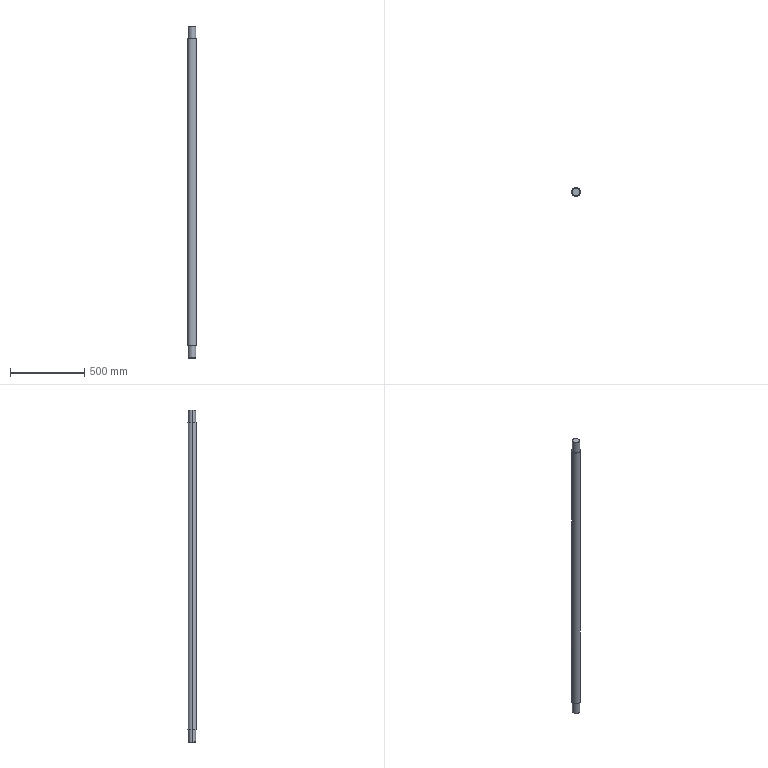Part | SolidWorks | features ICE 2, Chamfer 1, Extrusion 1, MirrorPattern 1 | 1 solid | 26 faces | box 60 x 60 x 2235 mm | volume 6164294 mm3 | cylinder 12 | plane 10 | cone 4 | commonest cylinder face diameters 14 x6 50 x4 60 x2
STEP:
#1=CARTESIAN_POINT('',(7.,24.,-1102.5));
#2=VERTEX_POINT('',#1);
#3=CARTESIAN_POINT('',(0.,25.,-1109.5));
#4=VERTEX_POINT('',#3);
#5=CARTESIAN_POINT('',(7.,24.,-1102.5));
#6=CARTESIAN_POINT('',(7.,24.,-1102.965));
#7=CARTESIAN_POINT('',(6.954,24.014,-1103.422));
#8=CARTESIAN_POINT('',(6.82,24.052,-1104.096));
#9=CARTESIAN_POINT('',(6.764,24.068,-1104.318));
#10=CARTESIAN_POINT('',(6.629,24.105,-1104.759));
#11=CARTESIAN_POINT('',(6.551,24.127,-1104.978));
#12=CARTESIAN_POINT('',(6.287,24.197,-1105.613));
#13=CARTESIAN_POINT('',(6.071,24.253,-1106.014));
#14=CARTESIAN_POINT('',(5.69,24.344,-1106.583));
#15=CARTESIAN_POINT('',(5.552,24.376,-1106.769));
#16=CARTESIAN_POINT('',(5.261,24.441,-1107.123));
#17=CARTESIAN_POINT('',(5.108,24.473,-1107.291));
#18=CARTESIAN_POINT('',(4.626,24.57,-1107.773));
#19=CARTESIAN_POINT('',(4.275,24.635,-1108.062));
#20=CARTESIAN_POINT('',(3.51,24.755,-1108.574));
#21=CARTESIAN_POINT('',(3.106,24.81,-1108.79));
#22=CARTESIAN_POINT('',(2.475,24.878,-1109.052));
#23=CARTESIAN_POINT('',(2.26,24.899,-1109.129));
#24=CARTESIAN_POINT('',(1.82,24.935,-1109.263));
#25=CARTESIAN_POINT('',(1.594,24.95,-1109.32));
#26=CARTESIAN_POINT('',(0.9153,24.987,-1109.455));
#27=CARTESIAN_POINT('',(0.4594,25.,-1109.5));
#28=CARTESIAN_POINT('',(0.,25.,-1109.5));
#29=B_SPLINE_CURVE_WITH_KNOTS('',3,(#5,#6,#7,#8,#9,#10,#11,#12,#13,#14,#15,#16,#17,#18,#19,#20,#21,#22,#23,#24,#25,#26,#27,#28),.UNSPECIFIED.,.F.,.F.,(4,2,2,2,2,2,2,2,2,2,2,4),(0.,0.001375,0.002063,0.00275,0.004125,0.004813,0.0055,0.006875,0.00825,0.008938,0.009626,0.011),.UNSPECIFIED.);
#30=EDGE_CURVE('',#2,#4,#29,.T.);
#31=ORIENTED_EDGE('',*,*,#30,.T.);
#32=CARTESIAN_POINT('',(0.,19.5,-1109.5));
#33=VERTEX_POINT('',#32);
#34=CARTESIAN_POINT('',(0.,25.,-1109.5));
#35=DIRECTION('',(0.,-1.,0.));
#36=VECTOR('',#35,1000.);
#37=LINE('',#34,#36);
#38=EDGE_CURVE('',#4,#33,#37,.T.);
#39=ORIENTED_EDGE('',*,*,#38,.T.);
#40=CARTESIAN_POINT('',(7.,19.5,-1102.5));
#41=VERTEX_POINT('',#40);
#42=CARTESIAN_POINT('',(0.,19.5,-1102.5));
#43=DIRECTION('',(0.,-1.,0.));
#44=DIRECTION('',(0.,0.,1.));
#45=AXIS2_PLACEMENT_3D('',#42,#43,#44);
#46=CIRCLE('',#45,7.);
#47=EDGE_CURVE('',#33,#41,#46,.T.);
#48=ORIENTED_EDGE('',*,*,#47,.T.);
#49=CARTESIAN_POINT('',(7.,25.,-1102.5));
#50=DIRECTION('',(0.,-1.,0.));
#51=VECTOR('',#50,1000.);
#52=LINE('',#49,#51);
#53=EDGE_CURVE('',#2,#41,#52,.T.);
#54=ORIENTED_EDGE('',*,*,#53,.F.);
#55=EDGE_LOOP('',(#31,#39,#48,#54));
#56=FACE_OUTER_BOUND('',#55,.T.);
#57=CARTESIAN_POINT('',(0.,25.,-1102.5));
#58=DIRECTION('',(0.,-1.,0.));
#59=DIRECTION('',(0.,0.,-1.));
#60=AXIS2_PLACEMENT_3D('',#57,#58,#59);
#61=CYLINDRICAL_SURFACE('',#60,7.);
#62=ADVANCED_FACE('',(#56),#61,.F.);
#63=CARTESIAN_POINT('',(-24.,0.,-1117.5));
#64=VERTEX_POINT('',#63);
#65=CARTESIAN_POINT('',(24.,0.,-1117.5));
#66=VERTEX_POINT('',#65);
#67=CARTESIAN_POINT('',(0.,0.,-1117.5));
#68=DIRECTION('',(0.,0.,-1.));
#69=DIRECTION('',(-1.,0.,0.));
#70=AXIS2_PLACEMENT_3D('',#67,#68,#69);
#71=CIRCLE('',#70,24.);
#72=EDGE_CURVE('',#64,#66,#71,.T.);
#73=ORIENTED_EDGE('',*,*,#72,.F.);
#74=CARTESIAN_POINT('',(-25.,0.,-1116.5));
#75=VERTEX_POINT('',#74);
#76=CARTESIAN_POINT('',(-25.,0.,-1116.5));
#77=DIRECTION('',(-0.7071,0.,0.7071));
#78=VECTOR('',#77,1000.);
#79=LINE('',#76,#78);
#80=EDGE_CURVE('',#64,#75,#79,.T.);
#81=ORIENTED_EDGE('',*,*,#80,.T.);
#82=CARTESIAN_POINT('',(25.,0.,-1116.5));
#83=VERTEX_POINT('',#82);
#84=CARTESIAN_POINT('',(0.,0.,-1116.5));
#85=DIRECTION('',(0.,0.,1.));
#86=DIRECTION('',(-1.,0.,0.));
#87=AXIS2_PLACEMENT_3D('',#84,#85,#86);
#88=CIRCLE('',#87,25.);
#89=EDGE_CURVE('',#83,#75,#88,.T.);
#90=ORIENTED_EDGE('',*,*,#89,.F.);
#91=CARTESIAN_POINT('',(25.,0.,-1116.5));
#92=DIRECTION('',(0.7071,0.,0.7071));
#93=VECTOR('',#92,1000.);
#94=LINE('',#91,#93);
#95=EDGE_CURVE('',#66,#83,#94,.T.);
#96=ORIENTED_EDGE('',*,*,#95,.F.);
#97=EDGE_LOOP('',(#73,#81,#90,#96));
#98=FACE_OUTER_BOUND('',#97,.T.);
#99=CARTESIAN_POINT('',(0.,0.,-1116.5));
#100=DIRECTION('',(0.,0.,1.));
#101=DIRECTION('',(1.,0.,0.));
#102=AXIS2_PLACEMENT_3D('',#99,#100,#101);
#103=CONICAL_SURFACE('',#102,25.,0.7854);
#104=ADVANCED_FACE('',(#98),#103,.T.);
#105=ORIENTED_EDGE('',*,*,#30,.F.);
#106=CARTESIAN_POINT('',(7.,24.,-1046.5));
#107=VERTEX_POINT('',#106);
#108=CARTESIAN_POINT('',(7.,24.,-1117.5));
#109=DIRECTION('',(0.,0.,-1.));
#110=VECTOR('',#109,1000.);
#111=LINE('',#108,#110);
#112=EDGE_CURVE('',#107,#2,#111,.T.);
#113=ORIENTED_EDGE('',*,*,#112,.F.);
#114=CARTESIAN_POINT('',(-7.,24.,-1046.5));
#115=VERTEX_POINT('',#114);
#116=CARTESIAN_POINT('',(-7.,24.,-1046.5));
#117=CARTESIAN_POINT('',(-7.,24.,-1046.035));
#118=CARTESIAN_POINT('',(-6.954,24.014,-1045.579));
#119=CARTESIAN_POINT('',(-6.82,24.052,-1044.905));
#120=CARTESIAN_POINT('',(-6.764,24.068,-1044.683));
#121=CARTESIAN_POINT('',(-6.63,24.105,-1044.242));
#122=CARTESIAN_POINT('',(-6.551,24.126,-1044.024));
#123=CARTESIAN_POINT('',(-6.287,24.197,-1043.389));
#124=CARTESIAN_POINT('',(-6.072,24.253,-1042.988));
#125=CARTESIAN_POINT('',(-5.692,24.344,-1042.419));
#126=CARTESIAN_POINT('',(-5.554,24.376,-1042.233));
#127=CARTESIAN_POINT('',(-5.263,24.44,-1041.88));
#128=CARTESIAN_POINT('',(-5.11,24.473,-1041.711));
#129=CARTESIAN_POINT('',(-4.629,24.57,-1041.229));
#130=CARTESIAN_POINT('',(-4.278,24.634,-1040.94));
#131=CARTESIAN_POINT('',(-3.514,24.755,-1040.429));
#132=CARTESIAN_POINT('',(-3.11,24.809,-1040.213));
#133=CARTESIAN_POINT('',(-2.48,24.878,-1039.95));
#134=CARTESIAN_POINT('',(-2.265,24.898,-1039.873));
#135=CARTESIAN_POINT('',(-1.825,24.934,-1039.738));
#136=CARTESIAN_POINT('',(-1.6,24.95,-1039.681));
#137=CARTESIAN_POINT('',(-0.9213,24.987,-1039.546));
#138=CARTESIAN_POINT('',(-0.4657,25.,-1039.5));
#139=CARTESIAN_POINT('',(0.4524,25.,-1039.5));
#140=CARTESIAN_POINT('',(0.9188,24.987,-1039.545));
#141=CARTESIAN_POINT('',(1.818,24.938,-1039.725));
#142=CARTESIAN_POINT('',(2.256,24.902,-1039.858));
#143=CARTESIAN_POINT('',(2.894,24.833,-1040.122));
#144=CARTESIAN_POINT('',(3.103,24.808,-1040.221));
#145=CARTESIAN_POINT('',(3.506,24.754,-1040.437));
#146=CARTESIAN_POINT('',(3.701,24.725,-1040.554));
#147=CARTESIAN_POINT('',(4.079,24.666,-1040.807));
#148=CARTESIAN_POINT('',(4.262,24.635,-1040.942));
#149=CARTESIAN_POINT('',(4.615,24.571,-1041.232));
#150=CARTESIAN_POINT('',(4.786,24.538,-1041.387));
#151=CARTESIAN_POINT('',(5.272,24.44,-1041.872));
#152=CARTESIAN_POINT('',(5.56,24.375,-1042.222));
#153=CARTESIAN_POINT('',(6.067,24.254,-1042.978));
#154=CARTESIAN_POINT('',(6.287,24.197,-1043.388));
#155=CARTESIAN_POINT('',(6.638,24.103,-1044.231));
#156=CARTESIAN_POINT('',(6.772,24.066,-1044.668));
#157=CARTESIAN_POINT('',(6.908,24.027,-1045.344));
#158=CARTESIAN_POINT('',(6.942,24.017,-1045.575));
#159=CARTESIAN_POINT('',(6.988,24.003,-1046.036));
#160=CARTESIAN_POINT('',(7.,24.,-1046.268));
#161=CARTESIAN_POINT('',(7.,24.,-1046.5));
#162=B_SPLINE_CURVE_WITH_KNOTS('',3,(#116,#117,#118,#119,#120,#121,#122,#123,#124,#125,#126,#127,#128,#129,#130,#131,#132,#133,#134,#135,#136,#137,#138,#139,#140,#141,#142,#143,#144,#145,#146,#147,#148,#149,#150,#151,#152,#153,#154,#155,#156,#157,#158,#159,#160,#161),.UNSPECIFIED.,.F.,.F.,(4,2,2,2,2,2,2,2,2,2,2,2,2,2,2,2,2,2,2,2,2,2,4),(0.,0.001374,0.002061,0.002749,0.004123,0.00481,0.005497,0.006871,0.008246,0.008933,0.00962,0.01099,0.01237,0.01374,0.01443,0.01512,0.0158,0.01649,0.01787,0.01924,0.02061,0.0213,0.02199),.UNSPECIFIED.);
#163=EDGE_CURVE('',#115,#107,#162,.T.);
#164=ORIENTED_EDGE('',*,*,#163,.F.);
#165=CARTESIAN_POINT('',(-7.,24.,-1102.5));
#166=VERTEX_POINT('',#165);
#167=CARTESIAN_POINT('',(-7.,24.,-1117.5));
#168=DIRECTION('',(0.,0.,1.));
#169=VECTOR('',#168,1000.);
#170=LINE('',#167,#169);
#171=EDGE_CURVE('',#166,#115,#170,.T.);
#172=ORIENTED_EDGE('',*,*,#171,.F.);
#173=CARTESIAN_POINT('',(0.,25.,-1109.5));
#174=CARTESIAN_POINT('',(-0.4588,25.,-1109.5));
#175=CARTESIAN_POINT('',(-0.9249,24.987,-1109.454));
#176=CARTESIAN_POINT('',(-1.824,24.937,-1109.274));
#177=CARTESIAN_POINT('',(-2.261,24.901,-1109.141));
#178=CARTESIAN_POINT('',(-2.898,24.832,-1108.876));
#179=CARTESIAN_POINT('',(-3.107,24.807,-1108.777));
#180=CARTESIAN_POINT('',(-3.51,24.753,-1108.561));
#181=CARTESIAN_POINT('',(-3.705,24.725,-1108.443));
#182=CARTESIAN_POINT('',(-4.083,24.665,-1108.191));
#183=CARTESIAN_POINT('',(-4.265,24.634,-1108.055));
#184=CARTESIAN_POINT('',(-4.618,24.57,-1107.766));
#185=CARTESIAN_POINT('',(-4.789,24.538,-1107.611));
#186=CARTESIAN_POINT('',(-5.274,24.44,-1107.126));
#187=CARTESIAN_POINT('',(-5.561,24.375,-1106.775));
#188=CARTESIAN_POINT('',(-6.068,24.254,-1106.02));
#189=CARTESIAN_POINT('',(-6.288,24.197,-1105.61));
#190=CARTESIAN_POINT('',(-6.638,24.103,-1104.767));
#191=CARTESIAN_POINT('',(-6.772,24.066,-1104.331));
#192=CARTESIAN_POINT('',(-6.908,24.027,-1103.655));
#193=CARTESIAN_POINT('',(-6.943,24.017,-1103.425));
#194=CARTESIAN_POINT('',(-6.988,24.003,-1102.964));
#195=CARTESIAN_POINT('',(-7.,24.,-1102.732));
#196=CARTESIAN_POINT('',(-7.,24.,-1102.5));
#197=B_SPLINE_CURVE_WITH_KNOTS('',3,(#173,#174,#175,#176,#177,#178,#179,#180,#181,#182,#183,#184,#185,#186,#187,#188,#189,#190,#191,#192,#193,#194,#195,#196),.UNSPECIFIED.,.F.,.F.,(4,2,2,2,2,2,2,2,2,2,2,4),(0.011,0.01237,0.01375,0.01443,0.01512,0.01581,0.01649,0.01787,0.01924,0.02061,0.0213,0.02199),.UNSPECIFIED.);
#198=EDGE_CURVE('',#4,#166,#197,.T.);
#199=ORIENTED_EDGE('',*,*,#198,.F.);
#200=EDGE_LOOP('',(#105,#113,#164,#172,#199));
#201=FACE_BOUND('',#200,.T.);
#202=ORIENTED_EDGE('',*,*,#89,.T.);
#203=CARTESIAN_POINT('',(-25.,0.,-1033.5));
#204=VERTEX_POINT('',#203);
#205=CARTESIAN_POINT('',(-25.,0.,-1117.5));
#206=DIRECTION('',(0.,0.,1.));
#207=VECTOR('',#206,1000.);
#208=LINE('',#205,#207);
#209=EDGE_CURVE('',#75,#204,#208,.T.);
#210=ORIENTED_EDGE('',*,*,#209,.T.);
#211=CARTESIAN_POINT('',(25.,0.,-1033.5));
#212=VERTEX_POINT('',#211);
#213=CARTESIAN_POINT('',(0.,0.,-1033.5));
#214=DIRECTION('',(0.,0.,1.));
#215=DIRECTION('',(1.,0.,0.));
#216=AXIS2_PLACEMENT_3D('',#213,#214,#215);
#217=CIRCLE('',#216,25.);
#218=EDGE_CURVE('',#212,#204,#217,.T.);
#219=ORIENTED_EDGE('',*,*,#218,.F.);
#220=CARTESIAN_POINT('',(25.,0.,-1117.5));
#221=DIRECTION('',(0.,0.,1.));
#222=VECTOR('',#221,1000.);
#223=LINE('',#220,#222);
#224=EDGE_CURVE('',#83,#212,#223,.T.);
#225=ORIENTED_EDGE('',*,*,#224,.F.);
#226=EDGE_LOOP('',(#202,#210,#219,#225));
#227=FACE_OUTER_BOUND('',#226,.T.);
#228=CARTESIAN_POINT('',(0.,0.,-1117.5));
#229=DIRECTION('',(0.,0.,1.));
#230=DIRECTION('',(1.,0.,0.));
#231=AXIS2_PLACEMENT_3D('',#228,#229,#230);
#232=CYLINDRICAL_SURFACE('',#231,25.);
#233=ADVANCED_FACE('',(#201,#227),#232,.T.);
#234=CARTESIAN_POINT('',(7.,24.,1046.5));
#235=VERTEX_POINT('',#234);
#236=CARTESIAN_POINT('',(0.,25.,1039.5));
#237=VERTEX_POINT('',#236);
#238=CARTESIAN_POINT('',(7.,24.,1046.5));
#239=CARTESIAN_POINT('',(7.,24.,1046.035));
#240=CARTESIAN_POINT('',(6.954,24.014,1045.578));
#241=CARTESIAN_POINT('',(6.82,24.052,1044.904));
#242=CARTESIAN_POINT('',(6.764,24.068,1044.682));
#243=CARTESIAN_POINT('',(6.629,24.105,1044.241));
#244=CARTESIAN_POINT('',(6.551,24.127,1044.022));
#245=CARTESIAN_POINT('',(6.287,24.197,1043.387));
#246=CARTESIAN_POINT('',(6.071,24.253,1042.986));
#247=CARTESIAN_POINT('',(5.69,24.344,1042.417));
#248=CARTESIAN_POINT('',(5.552,24.376,1042.231));
#249=CARTESIAN_POINT('',(5.261,24.441,1041.877));
#250=CARTESIAN_POINT('',(5.108,24.473,1041.709));
#251=CARTESIAN_POINT('',(4.626,24.57,1041.227));
#252=CARTESIAN_POINT('',(4.275,24.635,1040.938));
#253=CARTESIAN_POINT('',(3.51,24.755,1040.426));
#254=CARTESIAN_POINT('',(3.106,24.81,1040.21));
#255=CARTESIAN_POINT('',(2.475,24.878,1039.948));
#256=CARTESIAN_POINT('',(2.26,24.899,1039.871));
#257=CARTESIAN_POINT('',(1.82,24.935,1039.737));
#258=CARTESIAN_POINT('',(1.594,24.95,1039.68));
#259=CARTESIAN_POINT('',(0.9153,24.987,1039.545));
#260=CARTESIAN_POINT('',(0.4594,25.,1039.5));
#261=CARTESIAN_POINT('',(0.,25.,1039.5));
#262=B_SPLINE_CURVE_WITH_KNOTS('',3,(#238,#239,#240,#241,#242,#243,#244,#245,#246,#247,#248,#249,#250,#251,#252,#253,#254,#255,#256,#257,#258,#259,#260,#261),.UNSPECIFIED.,.F.,.F.,(4,2,2,2,2,2,2,2,2,2,2,4),(0.,0.001375,0.002063,0.00275,0.004125,0.004813,0.0055,0.006875,0.00825,0.008938,0.009626,0.011),.UNSPECIFIED.);
#263=EDGE_CURVE('',#235,#237,#262,.T.);
#264=ORIENTED_EDGE('',*,*,#263,.T.);
#265=CARTESIAN_POINT('',(0.,19.5,1039.5));
#266=VERTEX_POINT('',#265);
#267=CARTESIAN_POINT('',(0.,25.,1039.5));
#268=DIRECTION('',(0.,-1.,0.));
#269=VECTOR('',#268,1000.);
#270=LINE('',#267,#269);
#271=EDGE_CURVE('',#237,#266,#270,.T.);
#272=ORIENTED_EDGE('',*,*,#271,.T.);
#273=CARTESIAN_POINT('',(7.,19.5,1046.5));
#274=VERTEX_POINT('',#273);
#275=CARTESIAN_POINT('',(0.,19.5,1046.5));
#276=DIRECTION('',(0.,1.,0.));
#277=DIRECTION('',(0.,0.,-1.));
#278=AXIS2_PLACEMENT_3D('',#275,#276,#277);
#279=CIRCLE('',#278,7.);
#280=EDGE_CURVE('',#274,#266,#279,.T.);
#281=ORIENTED_EDGE('',*,*,#280,.F.);
#282=CARTESIAN_POINT('',(7.,25.,1046.5));
#283=DIRECTION('',(0.,-1.,0.));
#284=VECTOR('',#283,1000.);
#285=LINE('',#282,#284);
#286=EDGE_CURVE('',#235,#274,#285,.T.);
#287=ORIENTED_EDGE('',*,*,#286,.F.);
#288=EDGE_LOOP('',(#264,#272,#281,#287));
#289=FACE_OUTER_BOUND('',#288,.T.);
#290=CARTESIAN_POINT('',(0.,25.,1046.5));
#291=DIRECTION('',(0.,-1.,0.));
#292=DIRECTION('',(0.,0.,-1.));
#293=AXIS2_PLACEMENT_3D('',#290,#291,#292);
#294=CYLINDRICAL_SURFACE('',#293,7.);
#295=ADVANCED_FACE('',(#289),#294,.F.);
#296=CARTESIAN_POINT('',(24.,0.,1117.5));
#297=VERTEX_POINT('',#296);
#298=CARTESIAN_POINT('',(-24.,0.,1117.5));
#299=VERTEX_POINT('',#298);
#300=CARTESIAN_POINT('',(0.,0.,1117.5));
#301=DIRECTION('',(0.,0.,1.));
#302=DIRECTION('',(1.,0.,0.));
#303=AXIS2_PLACEMENT_3D('',#300,#301,#302);
#304=CIRCLE('',#303,24.);
#305=EDGE_CURVE('',#297,#299,#304,.T.);
#306=ORIENTED_EDGE('',*,*,#305,.F.);
#307=CARTESIAN_POINT('',(25.,0.,1116.5));
#308=VERTEX_POINT('',#307);
#309=CARTESIAN_POINT('',(24.,0.,1117.5));
#310=DIRECTION('',(0.7071,0.,-0.7071));
#311=VECTOR('',#310,1000.);
#312=LINE('',#309,#311);
#313=EDGE_CURVE('',#297,#308,#312,.T.);
#314=ORIENTED_EDGE('',*,*,#313,.T.);
#315=CARTESIAN_POINT('',(-25.,0.,1116.5));
#316=VERTEX_POINT('',#315);
#317=CARTESIAN_POINT('',(0.,0.,1116.5));
#318=DIRECTION('',(0.,0.,-1.));
#319=DIRECTION('',(1.,0.,0.));
#320=AXIS2_PLACEMENT_3D('',#317,#318,#319);
#321=CIRCLE('',#320,25.);
#322=EDGE_CURVE('',#316,#308,#321,.T.);
#323=ORIENTED_EDGE('',*,*,#322,.F.);
#324=CARTESIAN_POINT('',(-24.,0.,1117.5));
#325=DIRECTION('',(-0.7071,0.,-0.7071));
#326=VECTOR('',#325,1000.);
#327=LINE('',#324,#326);
#328=EDGE_CURVE('',#299,#316,#327,.T.);
#329=ORIENTED_EDGE('',*,*,#328,.F.);
#330=EDGE_LOOP('',(#306,#314,#323,#329));
#331=FACE_OUTER_BOUND('',#330,.T.);
#332=CARTESIAN_POINT('',(0.,0.,1117.5));
#333=DIRECTION('',(0.,0.,-1.));
#334=DIRECTION('',(-1.,0.,0.));
#335=AXIS2_PLACEMENT_3D('',#332,#333,#334);
#336=CONICAL_SURFACE('',#335,24.,0.7854);
#337=ADVANCED_FACE('',(#331),#336,.T.);
#338=CARTESIAN_POINT('',(30.,0.,1033.5));
#339=VERTEX_POINT('',#338);
#340=CARTESIAN_POINT('',(-30.,0.,1033.5));
#341=VERTEX_POINT('',#340);
#342=CARTESIAN_POINT('',(0.,0.,1033.5));
#343=DIRECTION('',(0.,0.,1.));
#344=DIRECTION('',(1.,0.,0.));
#345=AXIS2_PLACEMENT_3D('',#342,#343,#344);
#346=CIRCLE('',#345,30.);
#347=EDGE_CURVE('',#339,#341,#346,.T.);
#348=ORIENTED_EDGE('',*,*,#347,.F.);
#349=CARTESIAN_POINT('',(30.,0.,-1033.5));
#350=VERTEX_POINT('',#349);
#351=CARTESIAN_POINT('',(30.,0.,1033.5));
#352=DIRECTION('',(0.,0.,-1.));
#353=VECTOR('',#352,1000.);
#354=LINE('',#351,#353);
#355=EDGE_CURVE('',#339,#350,#354,.T.);
#356=ORIENTED_EDGE('',*,*,#355,.T.);
#357=CARTESIAN_POINT('',(-30.,0.,-1033.5));
#358=VERTEX_POINT('',#357);
#359=CARTESIAN_POINT('',(0.,0.,-1033.5));
#360=DIRECTION('',(0.,0.,1.));
#361=DIRECTION('',(1.,0.,0.));
#362=AXIS2_PLACEMENT_3D('',#359,#360,#361);
#363=CIRCLE('',#362,30.);
#364=EDGE_CURVE('',#350,#358,#363,.T.);
#365=ORIENTED_EDGE('',*,*,#364,.T.);
#366=CARTESIAN_POINT('',(-30.,0.,1033.5));
#367=DIRECTION('',(0.,0.,-1.));
#368=VECTOR('',#367,1000.);
#369=LINE('',#366,#368);
#370=EDGE_CURVE('',#341,#358,#369,.T.);
#371=ORIENTED_EDGE('',*,*,#370,.F.);
#372=EDGE_LOOP('',(#348,#356,#365,#371));
#373=FACE_OUTER_BOUND('',#372,.T.);
#374=CARTESIAN_POINT('',(0.,0.,1033.5));
#375=DIRECTION('',(0.,0.,-1.));
#376=DIRECTION('',(-1.,0.,0.));
#377=AXIS2_PLACEMENT_3D('',#374,#375,#376);
#378=CYLINDRICAL_SURFACE('',#377,30.);
#379=ADVANCED_FACE('',(#373),#378,.T.);
#380=CARTESIAN_POINT('',(-7.,24.,1102.5));
#381=VERTEX_POINT('',#380);
#382=CARTESIAN_POINT('',(7.,24.,1102.5));
#383=VERTEX_POINT('',#382);
#384=CARTESIAN_POINT('',(-7.,24.,1102.5));
#385=CARTESIAN_POINT('',(-7.,24.,1102.965));
#386=CARTESIAN_POINT('',(-6.954,24.014,1103.421));
#387=CARTESIAN_POINT('',(-6.82,24.052,1104.095));
#388=CARTESIAN_POINT('',(-6.764,24.068,1104.317));
#389=CARTESIAN_POINT('',(-6.63,24.105,1104.758));
#390=CARTESIAN_POINT('',(-6.551,24.126,1104.976));
#391=CARTESIAN_POINT('',(-6.287,24.197,1105.611));
#392=CARTESIAN_POINT('',(-6.072,24.253,1106.012));
#393=CARTESIAN_POINT('',(-5.692,24.344,1106.581));
#394=CARTESIAN_POINT('',(-5.554,24.376,1106.767));
#395=CARTESIAN_POINT('',(-5.263,24.44,1107.12));
#396=CARTESIAN_POINT('',(-5.11,24.473,1107.289));
#397=CARTESIAN_POINT('',(-4.629,24.57,1107.771));
#398=CARTESIAN_POINT('',(-4.278,24.634,1108.06));
#399=CARTESIAN_POINT('',(-3.514,24.755,1108.571));
#400=CARTESIAN_POINT('',(-3.11,24.809,1108.787));
#401=CARTESIAN_POINT('',(-2.48,24.878,1109.05));
#402=CARTESIAN_POINT('',(-2.265,24.898,1109.127));
#403=CARTESIAN_POINT('',(-1.825,24.934,1109.262));
#404=CARTESIAN_POINT('',(-1.6,24.95,1109.319));
#405=CARTESIAN_POINT('',(-0.9213,24.987,1109.454));
#406=CARTESIAN_POINT('',(-0.4657,25.,1109.5));
#407=CARTESIAN_POINT('',(0.4524,25.,1109.5));
#408=CARTESIAN_POINT('',(0.9188,24.987,1109.455));
#409=CARTESIAN_POINT('',(1.818,24.938,1109.275));
#410=CARTESIAN_POINT('',(2.256,24.902,1109.142));
#411=CARTESIAN_POINT('',(2.894,24.833,1108.878));
#412=CARTESIAN_POINT('',(3.103,24.808,1108.779));
#413=CARTESIAN_POINT('',(3.506,24.754,1108.563));
#414=CARTESIAN_POINT('',(3.701,24.725,1108.446));
#415=CARTESIAN_POINT('',(4.079,24.666,1108.193));
#416=CARTESIAN_POINT('',(4.262,24.635,1108.058));
#417=CARTESIAN_POINT('',(4.615,24.571,1107.768));
#418=CARTESIAN_POINT('',(4.786,24.538,1107.613));
#419=CARTESIAN_POINT('',(5.272,24.44,1107.128));
#420=CARTESIAN_POINT('',(5.56,24.375,1106.778));
#421=CARTESIAN_POINT('',(6.067,24.254,1106.022));
#422=CARTESIAN_POINT('',(6.287,24.197,1105.612));
#423=CARTESIAN_POINT('',(6.638,24.103,1104.769));
#424=CARTESIAN_POINT('',(6.772,24.066,1104.332));
#425=CARTESIAN_POINT('',(6.908,24.027,1103.656));
#426=CARTESIAN_POINT('',(6.942,24.017,1103.425));
#427=CARTESIAN_POINT('',(6.988,24.003,1102.964));
#428=CARTESIAN_POINT('',(7.,24.,1102.732));
#429=CARTESIAN_POINT('',(7.,24.,1102.5));
#430=B_SPLINE_CURVE_WITH_KNOTS('',3,(#384,#385,#386,#387,#388,#389,#390,#391,#392,#393,#394,#395,#396,#397,#398,#399,#400,#401,#402,#403,#404,#405,#406,#407,#408,#409,#410,#411,#412,#413,#414,#415,#416,#417,#418,#419,#420,#421,#422,#423,#424,#425,#426,#427,#428,#429),.UNSPECIFIED.,.F.,.F.,(4,2,2,2,2,2,2,2,2,2,2,2,2,2,2,2,2,2,2,2,2,2,4),(0.,0.001374,0.002061,0.002749,0.004123,0.00481,0.005497,0.006871,0.008246,0.008933,0.00962,0.01099,0.01237,0.01374,0.01443,0.01512,0.0158,0.01649,0.01787,0.01924,0.02061,0.0213,0.02199),.UNSPECIFIED.);
#431=EDGE_CURVE('',#381,#383,#430,.T.);
#432=ORIENTED_EDGE('',*,*,#431,.F.);
#433=CARTESIAN_POINT('',(-7.,24.,1046.5));
#434=VERTEX_POINT('',#433);
#435=CARTESIAN_POINT('',(-7.,24.,1117.5));
#436=DIRECTION('',(0.,0.,1.));
#437=VECTOR('',#436,1000.);
#438=LINE('',#435,#437);
#439=EDGE_CURVE('',#434,#381,#438,.T.);
#440=ORIENTED_EDGE('',*,*,#439,.F.);
#441=CARTESIAN_POINT('',(0.,25.,1039.5));
#442=CARTESIAN_POINT('',(-0.4588,25.,1039.5));
#443=CARTESIAN_POINT('',(-0.9249,24.987,1039.546));
#444=CARTESIAN_POINT('',(-1.824,24.937,1039.726));
#445=CARTESIAN_POINT('',(-2.261,24.901,1039.859));
#446=CARTESIAN_POINT('',(-2.898,24.832,1040.124));
#447=CARTESIAN_POINT('',(-3.107,24.807,1040.223));
#448=CARTESIAN_POINT('',(-3.51,24.753,1040.439));
#449=CARTESIAN_POINT('',(-3.705,24.725,1040.557));
#450=CARTESIAN_POINT('',(-4.083,24.665,1040.809));
#451=CARTESIAN_POINT('',(-4.265,24.634,1040.945));
#452=CARTESIAN_POINT('',(-4.618,24.57,1041.234));
#453=CARTESIAN_POINT('',(-4.789,24.538,1041.389));
#454=CARTESIAN_POINT('',(-5.274,24.44,1041.874));
#455=CARTESIAN_POINT('',(-5.561,24.375,1042.225));
#456=CARTESIAN_POINT('',(-6.068,24.254,1042.98));
#457=CARTESIAN_POINT('',(-6.288,24.197,1043.39));
#458=CARTESIAN_POINT('',(-6.638,24.103,1044.233));
#459=CARTESIAN_POINT('',(-6.772,24.066,1044.669));
#460=CARTESIAN_POINT('',(-6.908,24.027,1045.345));
#461=CARTESIAN_POINT('',(-6.943,24.017,1045.575));
#462=CARTESIAN_POINT('',(-6.988,24.003,1046.036));
#463=CARTESIAN_POINT('',(-7.,24.,1046.268));
#464=CARTESIAN_POINT('',(-7.,24.,1046.5));
#465=B_SPLINE_CURVE_WITH_KNOTS('',3,(#441,#442,#443,#444,#445,#446,#447,#448,#449,#450,#451,#452,#453,#454,#455,#456,#457,#458,#459,#460,#461,#462,#463,#464),.UNSPECIFIED.,.F.,.F.,(4,2,2,2,2,2,2,2,2,2,2,4),(0.011,0.01237,0.01375,0.01443,0.01512,0.01581,0.01649,0.01787,0.01924,0.02061,0.0213,0.02199),.UNSPECIFIED.);
#466=EDGE_CURVE('',#237,#434,#465,.T.);
#467=ORIENTED_EDGE('',*,*,#466,.F.);
#468=ORIENTED_EDGE('',*,*,#263,.F.);
#469=CARTESIAN_POINT('',(7.,24.,1117.5));
#470=DIRECTION('',(0.,0.,-1.));
#471=VECTOR('',#470,1000.);
#472=LINE('',#469,#471);
#473=EDGE_CURVE('',#383,#235,#472,.T.);
#474=ORIENTED_EDGE('',*,*,#473,.F.);
#475=EDGE_LOOP('',(#432,#440,#467,#468,#474));
#476=FACE_BOUND('',#475,.T.);
#477=ORIENTED_EDGE('',*,*,#322,.T.);
#478=CARTESIAN_POINT('',(25.,0.,1033.5));
#479=VERTEX_POINT('',#478);
#480=CARTESIAN_POINT('',(25.,0.,1117.5));
#481=DIRECTION('',(0.,0.,-1.));
#482=VECTOR('',#481,1000.);
#483=LINE('',#480,#482);
#484=EDGE_CURVE('',#308,#479,#483,.T.);
#485=ORIENTED_EDGE('',*,*,#484,.T.);
#486=CARTESIAN_POINT('',(-25.,0.,1033.5));
#487=VERTEX_POINT('',#486);
#488=CARTESIAN_POINT('',(0.,0.,1033.5));
#489=DIRECTION('',(0.,0.,1.));
#490=DIRECTION('',(1.,0.,0.));
#491=AXIS2_PLACEMENT_3D('',#488,#489,#490);
#492=CIRCLE('',#491,25.);
#493=EDGE_CURVE('',#479,#487,#492,.T.);
#494=ORIENTED_EDGE('',*,*,#493,.T.);
#495=CARTESIAN_POINT('',(-25.,0.,1117.5));
#496=DIRECTION('',(0.,0.,-1.));
#497=VECTOR('',#496,1000.);
#498=LINE('',#495,#497);
#499=EDGE_CURVE('',#316,#487,#498,.T.);
#500=ORIENTED_EDGE('',*,*,#499,.F.);
#501=EDGE_LOOP('',(#477,#485,#494,#500));
#502=FACE_OUTER_BOUND('',#501,.T.);
#503=CARTESIAN_POINT('',(0.,0.,1117.5));
#504=DIRECTION('',(0.,0.,-1.));
#505=DIRECTION('',(-1.,0.,0.));
#506=AXIS2_PLACEMENT_3D('',#503,#504,#505);
#507=CYLINDRICAL_SURFACE('',#506,25.);
#508=ADVANCED_FACE('',(#476,#502),#507,.T.);
#509=ORIENTED_EDGE('',*,*,#484,.F.);
#510=CARTESIAN_POINT('',(0.,0.,1116.5));
#511=DIRECTION('',(0.,0.,-1.));
#512=DIRECTION('',(1.,0.,0.));
#513=AXIS2_PLACEMENT_3D('',#510,#511,#512);
#514=CIRCLE('',#513,25.);
#515=EDGE_CURVE('',#308,#316,#514,.T.);
#516=ORIENTED_EDGE('',*,*,#515,.T.);
#517=ORIENTED_EDGE('',*,*,#499,.T.);
#518=CARTESIAN_POINT('',(0.,0.,1033.5));
#519=DIRECTION('',(0.,0.,1.));
#520=DIRECTION('',(1.,0.,0.));
#521=AXIS2_PLACEMENT_3D('',#518,#519,#520);
#522=CIRCLE('',#521,25.);
#523=EDGE_CURVE('',#487,#479,#522,.T.);
#524=ORIENTED_EDGE('',*,*,#523,.T.);
#525=EDGE_LOOP('',(#509,#516,#517,#524));
#526=FACE_OUTER_BOUND('',#525,.T.);
#527=CARTESIAN_POINT('',(0.,0.,1117.5));
#528=DIRECTION('',(0.,0.,-1.));
#529=DIRECTION('',(-1.,0.,0.));
#530=AXIS2_PLACEMENT_3D('',#527,#528,#529);
#531=CYLINDRICAL_SURFACE('',#530,25.);
#532=ADVANCED_FACE('',(#526),#531,.T.);
#533=CARTESIAN_POINT('',(0.,0.,1033.5));
#534=DIRECTION('',(0.,0.,1.));
#535=DIRECTION('',(1.,0.,0.));
#536=AXIS2_PLACEMENT_3D('',#533,#534,#535);
#537=CIRCLE('',#536,30.);
#538=EDGE_CURVE('',#341,#339,#537,.T.);
#539=ORIENTED_EDGE('',*,*,#538,.T.);
#540=ORIENTED_EDGE('',*,*,#347,.T.);
#541=EDGE_LOOP('',(#539,#540));
#542=FACE_OUTER_BOUND('',#541,.T.);
#543=ORIENTED_EDGE('',*,*,#523,.F.);
#544=ORIENTED_EDGE('',*,*,#493,.F.);
#545=EDGE_LOOP('',(#543,#544));
#546=FACE_BOUND('',#545,.T.);
#547=CARTESIAN_POINT('',(0.,0.,1033.5));
#548=DIRECTION('',(0.,0.,1.));
#549=DIRECTION('',(1.,0.,0.));
#550=AXIS2_PLACEMENT_3D('',#547,#548,#549);
#551=PLANE('',#550);
#552=ADVANCED_FACE('',(#542,#546),#551,.T.);
#553=ORIENTED_EDGE('',*,*,#355,.F.);
#554=ORIENTED_EDGE('',*,*,#538,.F.);
#555=ORIENTED_EDGE('',*,*,#370,.T.);
#556=CARTESIAN_POINT('',(0.,0.,-1033.5));
#557=DIRECTION('',(0.,0.,1.));
#558=DIRECTION('',(1.,0.,0.));
#559=AXIS2_PLACEMENT_3D('',#556,#557,#558);
#560=CIRCLE('',#559,30.);
#561=EDGE_CURVE('',#358,#350,#560,.T.);
#562=ORIENTED_EDGE('',*,*,#561,.T.);
#563=EDGE_LOOP('',(#553,#554,#555,#562));
#564=FACE_OUTER_BOUND('',#563,.T.);
#565=CARTESIAN_POINT('',(0.,0.,1033.5));
#566=DIRECTION('',(0.,0.,-1.));
#567=DIRECTION('',(-1.,0.,0.));
#568=AXIS2_PLACEMENT_3D('',#565,#566,#567);
#569=CYLINDRICAL_SURFACE('',#568,30.);
#570=ADVANCED_FACE('',(#564),#569,.T.);
#571=ORIENTED_EDGE('',*,*,#218,.T.);
#572=CARTESIAN_POINT('',(0.,0.,-1033.5));
#573=DIRECTION('',(0.,0.,1.));
#574=DIRECTION('',(1.,0.,0.));
#575=AXIS2_PLACEMENT_3D('',#572,#573,#574);
#576=CIRCLE('',#575,25.);
#577=EDGE_CURVE('',#204,#212,#576,.T.);
#578=ORIENTED_EDGE('',*,*,#577,.T.);
#579=EDGE_LOOP('',(#571,#578));
#580=FACE_BOUND('',#579,.T.);
#581=ORIENTED_EDGE('',*,*,#561,.F.);
#582=ORIENTED_EDGE('',*,*,#364,.F.);
#583=EDGE_LOOP('',(#581,#582));
#584=FACE_OUTER_BOUND('',#583,.T.);
#585=CARTESIAN_POINT('',(0.,0.,-1033.5));
#586=DIRECTION('',(0.,0.,1.));
#587=DIRECTION('',(1.,0.,0.));
#588=AXIS2_PLACEMENT_3D('',#585,#586,#587);
#589=PLANE('',#588);
#590=ADVANCED_FACE('',(#580,#584),#589,.F.);
#591=CARTESIAN_POINT('',(0.,0.,1117.5));
#592=DIRECTION('',(0.,0.,1.));
#593=DIRECTION('',(1.,0.,0.));
#594=AXIS2_PLACEMENT_3D('',#591,#592,#593);
#595=CIRCLE('',#594,24.);
#596=EDGE_CURVE('',#299,#297,#595,.T.);
#597=ORIENTED_EDGE('',*,*,#596,.T.);
#598=ORIENTED_EDGE('',*,*,#305,.T.);
#599=EDGE_LOOP('',(#597,#598));
#600=FACE_OUTER_BOUND('',#599,.T.);
#601=CARTESIAN_POINT('',(0.,0.,1117.5));
#602=DIRECTION('',(0.,0.,1.));
#603=DIRECTION('',(1.,0.,0.));
#604=AXIS2_PLACEMENT_3D('',#601,#602,#603);
#605=PLANE('',#604);
#606=ADVANCED_FACE('',(#600),#605,.T.);
#607=ORIENTED_EDGE('',*,*,#313,.F.);
#608=ORIENTED_EDGE('',*,*,#596,.F.);
#609=ORIENTED_EDGE('',*,*,#328,.T.);
#610=ORIENTED_EDGE('',*,*,#515,.F.);
#611=EDGE_LOOP('',(#607,#608,#609,#610));
#612=FACE_OUTER_BOUND('',#611,.T.);
#613=CARTESIAN_POINT('',(0.,0.,1117.5));
#614=DIRECTION('',(0.,0.,-1.));
#615=DIRECTION('',(-1.,0.,0.));
#616=AXIS2_PLACEMENT_3D('',#613,#614,#615);
#617=CONICAL_SURFACE('',#616,24.,0.7854);
#618=ADVANCED_FACE('',(#612),#617,.T.);
#619=ORIENTED_EDGE('',*,*,#271,.F.);
#620=ORIENTED_EDGE('',*,*,#466,.T.);
#621=CARTESIAN_POINT('',(-7.,19.5,1046.5));
#622=VERTEX_POINT('',#621);
#623=CARTESIAN_POINT('',(-7.,25.,1046.5));
#624=DIRECTION('',(0.,-1.,0.));
#625=VECTOR('',#624,1000.);
#626=LINE('',#623,#625);
#627=EDGE_CURVE('',#434,#622,#626,.T.);
#628=ORIENTED_EDGE('',*,*,#627,.T.);
#629=CARTESIAN_POINT('',(0.,19.5,1046.5));
#630=DIRECTION('',(0.,1.,0.));
#631=DIRECTION('',(0.,0.,-1.));
#632=AXIS2_PLACEMENT_3D('',#629,#630,#631);
#633=CIRCLE('',#632,7.);
#634=EDGE_CURVE('',#266,#622,#633,.T.);
#635=ORIENTED_EDGE('',*,*,#634,.F.);
#636=EDGE_LOOP('',(#619,#620,#628,#635));
#637=FACE_OUTER_BOUND('',#636,.T.);
#638=CARTESIAN_POINT('',(0.,25.,1046.5));
#639=DIRECTION('',(0.,-1.,0.));
#640=DIRECTION('',(0.,0.,-1.));
#641=AXIS2_PLACEMENT_3D('',#638,#639,#640);
#642=CYLINDRICAL_SURFACE('',#641,7.);
#643=ADVANCED_FACE('',(#637),#642,.F.);
#644=ORIENTED_EDGE('',*,*,#439,.T.);
#645=CARTESIAN_POINT('',(-7.,19.5,1102.5));
#646=VERTEX_POINT('',#645);
#647=CARTESIAN_POINT('',(-7.,25.,1102.5));
#648=DIRECTION('',(0.,-1.,0.));
#649=VECTOR('',#648,1000.);
#650=LINE('',#647,#649);
#651=EDGE_CURVE('',#381,#646,#650,.T.);
#652=ORIENTED_EDGE('',*,*,#651,.T.);
#653=CARTESIAN_POINT('',(-7.,19.5,1102.5));
#654=DIRECTION('',(0.,0.,1.));
#655=VECTOR('',#654,1000.);
#656=LINE('',#653,#655);
#657=EDGE_CURVE('',#622,#646,#656,.T.);
#658=ORIENTED_EDGE('',*,*,#657,.F.);
#659=ORIENTED_EDGE('',*,*,#627,.F.);
#660=EDGE_LOOP('',(#644,#652,#658,#659));
#661=FACE_OUTER_BOUND('',#660,.T.);
#662=CARTESIAN_POINT('',(-7.,25.,1102.5));
#663=DIRECTION('',(1.,0.,0.));
#664=DIRECTION('',(0.,0.,-1.));
#665=AXIS2_PLACEMENT_3D('',#662,#663,#664);
#666=PLANE('',#665);
#667=ADVANCED_FACE('',(#661),#666,.T.);
#668=ORIENTED_EDGE('',*,*,#651,.F.);
#669=ORIENTED_EDGE('',*,*,#431,.T.);
#670=CARTESIAN_POINT('',(7.,19.5,1102.5));
#671=VERTEX_POINT('',#670);
#672=CARTESIAN_POINT('',(7.,25.,1102.5));
#673=DIRECTION('',(0.,-1.,0.));
#674=VECTOR('',#673,1000.);
#675=LINE('',#672,#674);
#676=EDGE_CURVE('',#383,#671,#675,.T.);
#677=ORIENTED_EDGE('',*,*,#676,.T.);
#678=CARTESIAN_POINT('',(0.,19.5,1102.5));
#679=DIRECTION('',(0.,1.,0.));
#680=DIRECTION('',(0.,0.,-1.));
#681=AXIS2_PLACEMENT_3D('',#678,#679,#680);
#682=CIRCLE('',#681,7.);
#683=EDGE_CURVE('',#646,#671,#682,.T.);
#684=ORIENTED_EDGE('',*,*,#683,.F.);
#685=EDGE_LOOP('',(#668,#669,#677,#684));
#686=FACE_OUTER_BOUND('',#685,.T.);
#687=CARTESIAN_POINT('',(0.,25.,1102.5));
#688=DIRECTION('',(0.,-1.,0.));
#689=DIRECTION('',(0.,0.,-1.));
#690=AXIS2_PLACEMENT_3D('',#687,#688,#689);
#691=CYLINDRICAL_SURFACE('',#690,7.);
#692=ADVANCED_FACE('',(#686),#691,.F.);
#693=ORIENTED_EDGE('',*,*,#473,.T.);
#694=ORIENTED_EDGE('',*,*,#286,.T.);
#695=CARTESIAN_POINT('',(7.,19.5,1046.5));
#696=DIRECTION('',(0.,0.,-1.));
#697=VECTOR('',#696,1000.);
#698=LINE('',#695,#697);
#699=EDGE_CURVE('',#671,#274,#698,.T.);
#700=ORIENTED_EDGE('',*,*,#699,.F.);
#701=ORIENTED_EDGE('',*,*,#676,.F.);
#702=EDGE_LOOP('',(#693,#694,#700,#701));
#703=FACE_OUTER_BOUND('',#702,.T.);
#704=CARTESIAN_POINT('',(7.,25.,1046.5));
#705=DIRECTION('',(-1.,0.,0.));
#706=DIRECTION('',(0.,0.,1.));
#707=AXIS2_PLACEMENT_3D('',#704,#705,#706);
#708=PLANE('',#707);
#709=ADVANCED_FACE('',(#703),#708,.T.);
#710=ORIENTED_EDGE('',*,*,#280,.T.);
#711=ORIENTED_EDGE('',*,*,#634,.T.);
#712=ORIENTED_EDGE('',*,*,#657,.T.);
#713=ORIENTED_EDGE('',*,*,#683,.T.);
#714=ORIENTED_EDGE('',*,*,#699,.T.);
#715=EDGE_LOOP('',(#710,#711,#712,#713,#714));
#716=FACE_OUTER_BOUND('',#715,.T.);
#717=CARTESIAN_POINT('',(0.,19.5,1046.5));
#718=DIRECTION('',(0.,-1.,0.));
#719=DIRECTION('',(0.,0.,-1.));
#720=AXIS2_PLACEMENT_3D('',#717,#718,#719);
#721=PLANE('',#720);
#722=ADVANCED_FACE('',(#716),#721,.F.);
#723=ORIENTED_EDGE('',*,*,#209,.F.);
#724=CARTESIAN_POINT('',(0.,0.,-1116.5));
#725=DIRECTION('',(0.,0.,1.));
#726=DIRECTION('',(-1.,0.,0.));
#727=AXIS2_PLACEMENT_3D('',#724,#725,#726);
#728=CIRCLE('',#727,25.);
#729=EDGE_CURVE('',#75,#83,#728,.T.);
#730=ORIENTED_EDGE('',*,*,#729,.T.);
#731=ORIENTED_EDGE('',*,*,#224,.T.);
#732=ORIENTED_EDGE('',*,*,#577,.F.);
#733=EDGE_LOOP('',(#723,#730,#731,#732));
#734=FACE_OUTER_BOUND('',#733,.T.);
#735=CARTESIAN_POINT('',(0.,0.,-1117.5));
#736=DIRECTION('',(0.,0.,1.));
#737=DIRECTION('',(1.,0.,0.));
#738=AXIS2_PLACEMENT_3D('',#735,#736,#737);
#739=CYLINDRICAL_SURFACE('',#738,25.);
#740=ADVANCED_FACE('',(#734),#739,.T.);
#741=CARTESIAN_POINT('',(0.,0.,-1117.5));
#742=DIRECTION('',(0.,0.,-1.));
#743=DIRECTION('',(-1.,0.,0.));
#744=AXIS2_PLACEMENT_3D('',#741,#742,#743);
#745=CIRCLE('',#744,24.);
#746=EDGE_CURVE('',#66,#64,#745,.T.);
#747=ORIENTED_EDGE('',*,*,#746,.T.);
#748=ORIENTED_EDGE('',*,*,#72,.T.);
#749=EDGE_LOOP('',(#747,#748));
#750=FACE_OUTER_BOUND('',#749,.T.);
#751=CARTESIAN_POINT('',(0.,0.,-1117.5));
#752=DIRECTION('',(0.,0.,-1.));
#753=DIRECTION('',(1.,0.,0.));
#754=AXIS2_PLACEMENT_3D('',#751,#752,#753);
#755=PLANE('',#754);
#756=ADVANCED_FACE('',(#750),#755,.T.);
#757=ORIENTED_EDGE('',*,*,#80,.F.);
#758=ORIENTED_EDGE('',*,*,#746,.F.);
#759=ORIENTED_EDGE('',*,*,#95,.T.);
#760=ORIENTED_EDGE('',*,*,#729,.F.);
#761=EDGE_LOOP('',(#757,#758,#759,#760));
#762=FACE_OUTER_BOUND('',#761,.T.);
#763=CARTESIAN_POINT('',(0.,0.,-1116.5));
#764=DIRECTION('',(0.,0.,1.));
#765=DIRECTION('',(1.,0.,0.));
#766=AXIS2_PLACEMENT_3D('',#763,#764,#765);
#767=CONICAL_SURFACE('',#766,25.,0.7854);
#768=ADVANCED_FACE('',(#762),#767,.T.);
#769=CARTESIAN_POINT('',(-7.,19.5,-1046.5));
#770=VERTEX_POINT('',#769);
#771=CARTESIAN_POINT('',(-7.,25.,-1046.5));
#772=DIRECTION('',(0.,-1.,0.));
#773=VECTOR('',#772,1000.);
#774=LINE('',#771,#773);
#775=EDGE_CURVE('',#115,#770,#774,.T.);
#776=ORIENTED_EDGE('',*,*,#775,.F.);
#777=ORIENTED_EDGE('',*,*,#163,.T.);
#778=CARTESIAN_POINT('',(7.,19.5,-1046.5));
#779=VERTEX_POINT('',#778);
#780=CARTESIAN_POINT('',(7.,25.,-1046.5));
#781=DIRECTION('',(0.,-1.,0.));
#782=VECTOR('',#781,1000.);
#783=LINE('',#780,#782);
#784=EDGE_CURVE('',#107,#779,#783,.T.);
#785=ORIENTED_EDGE('',*,*,#784,.T.);
#786=CARTESIAN_POINT('',(0.,19.5,-1046.5));
#787=DIRECTION('',(0.,-1.,0.));
#788=DIRECTION('',(0.,0.,1.));
#789=AXIS2_PLACEMENT_3D('',#786,#787,#788);
#790=CIRCLE('',#789,7.);
#791=EDGE_CURVE('',#779,#770,#790,.T.);
#792=ORIENTED_EDGE('',*,*,#791,.T.);
#793=EDGE_LOOP('',(#776,#777,#785,#792));
#794=FACE_OUTER_BOUND('',#793,.T.);
#795=CARTESIAN_POINT('',(0.,25.,-1046.5));
#796=DIRECTION('',(0.,-1.,0.));
#797=DIRECTION('',(0.,0.,-1.));
#798=AXIS2_PLACEMENT_3D('',#795,#796,#797);
#799=CYLINDRICAL_SURFACE('',#798,7.);
#800=ADVANCED_FACE('',(#794),#799,.F.);
#801=ORIENTED_EDGE('',*,*,#112,.T.);
#802=ORIENTED_EDGE('',*,*,#53,.T.);
#803=CARTESIAN_POINT('',(7.,19.5,-1046.5));
#804=DIRECTION('',(0.,0.,1.));
#805=VECTOR('',#804,1000.);
#806=LINE('',#803,#805);
#807=EDGE_CURVE('',#41,#779,#806,.T.);
#808=ORIENTED_EDGE('',*,*,#807,.T.);
#809=ORIENTED_EDGE('',*,*,#784,.F.);
#810=EDGE_LOOP('',(#801,#802,#808,#809));
#811=FACE_OUTER_BOUND('',#810,.T.);
#812=CARTESIAN_POINT('',(7.,25.,-1046.5));
#813=DIRECTION('',(1.,0.,0.));
#814=DIRECTION('',(0.,0.,-1.));
#815=AXIS2_PLACEMENT_3D('',#812,#813,#814);
#816=PLANE('',#815);
#817=ADVANCED_FACE('',(#811),#816,.F.);
#818=ORIENTED_EDGE('',*,*,#38,.F.);
#819=ORIENTED_EDGE('',*,*,#198,.T.);
#820=CARTESIAN_POINT('',(-7.,19.5,-1102.5));
#821=VERTEX_POINT('',#820);
#822=CARTESIAN_POINT('',(-7.,25.,-1102.5));
#823=DIRECTION('',(0.,-1.,0.));
#824=VECTOR('',#823,1000.);
#825=LINE('',#822,#824);
#826=EDGE_CURVE('',#166,#821,#825,.T.);
#827=ORIENTED_EDGE('',*,*,#826,.T.);
#828=CARTESIAN_POINT('',(0.,19.5,-1102.5));
#829=DIRECTION('',(0.,-1.,0.));
#830=DIRECTION('',(0.,0.,1.));
#831=AXIS2_PLACEMENT_3D('',#828,#829,#830);
#832=CIRCLE('',#831,7.);
#833=EDGE_CURVE('',#821,#33,#832,.T.);
#834=ORIENTED_EDGE('',*,*,#833,.T.);
#835=EDGE_LOOP('',(#818,#819,#827,#834));
#836=FACE_OUTER_BOUND('',#835,.T.);
#837=CARTESIAN_POINT('',(0.,25.,-1102.5));
#838=DIRECTION('',(0.,-1.,0.));
#839=DIRECTION('',(0.,0.,-1.));
#840=AXIS2_PLACEMENT_3D('',#837,#838,#839);
#841=CYLINDRICAL_SURFACE('',#840,7.);
#842=ADVANCED_FACE('',(#836),#841,.F.);
#843=ORIENTED_EDGE('',*,*,#171,.T.);
#844=ORIENTED_EDGE('',*,*,#775,.T.);
#845=CARTESIAN_POINT('',(-7.,19.5,-1102.5));
#846=DIRECTION('',(0.,0.,-1.));
#847=VECTOR('',#846,1000.);
#848=LINE('',#845,#847);
#849=EDGE_CURVE('',#770,#821,#848,.T.);
#850=ORIENTED_EDGE('',*,*,#849,.T.);
#851=ORIENTED_EDGE('',*,*,#826,.F.);
#852=EDGE_LOOP('',(#843,#844,#850,#851));
#853=FACE_OUTER_BOUND('',#852,.T.);
#854=CARTESIAN_POINT('',(-7.,25.,-1102.5));
#855=DIRECTION('',(-1.,0.,0.));
#856=DIRECTION('',(0.,0.,1.));
#857=AXIS2_PLACEMENT_3D('',#854,#855,#856);
#858=PLANE('',#857);
#859=ADVANCED_FACE('',(#853),#858,.F.);
#860=ORIENTED_EDGE('',*,*,#791,.F.);
#861=ORIENTED_EDGE('',*,*,#807,.F.);
#862=ORIENTED_EDGE('',*,*,#47,.F.);
#863=ORIENTED_EDGE('',*,*,#833,.F.);
#864=ORIENTED_EDGE('',*,*,#849,.F.);
#865=EDGE_LOOP('',(#860,#861,#862,#863,#864));
#866=FACE_OUTER_BOUND('',#865,.T.);
#867=CARTESIAN_POINT('',(0.,19.5,-1046.5));
#868=DIRECTION('',(0.,-1.,0.));
#869=DIRECTION('',(0.,0.,1.));
#870=AXIS2_PLACEMENT_3D('',#867,#868,#869);
#871=PLANE('',#870);
#872=ADVANCED_FACE('',(#866),#871,.F.);
#873=CLOSED_SHELL('',(#62,#104,#233,#295,#337,#379,#508,#532,#552,#570,#590,#606,#618,#643,#667,#692,#709,#722,#740,#756,#768,#800,#817,#842,#859,#872));
#874=MANIFOLD_SOLID_BREP('',#873);
#875=CARTESIAN_POINT('',(0.,0.,0.));
#876=DIRECTION('',(0.,0.,1.));
#877=DIRECTION('',(1.,0.,0.));
#878=AXIS2_PLACEMENT_3D('',#875,#876,#877);
#879=(LENGTH_UNIT()NAMED_UNIT(*)SI_UNIT(.MILLI.,.METRE.));
#880=UNCERTAINTY_MEASURE_WITH_UNIT(LENGTH_MEASURE(0.00001),#879,'','');
#881=(NAMED_UNIT(*)PLANE_ANGLE_UNIT()SI_UNIT($,.RADIAN.));
#882=(NAMED_UNIT(*)SI_UNIT($,.STERADIAN.)SOLID_ANGLE_UNIT());
#883=(GEOMETRIC_REPRESENTATION_CONTEXT(3)GLOBAL_UNCERTAINTY_ASSIGNED_CONTEXT((#880))GLOBAL_UNIT_ASSIGNED_CONTEXT((#879,#881,#882))REPRESENTATION_CONTEXT('',''));
#884=ADVANCED_BREP_SHAPE_REPRESENTATION('',(#874,#878),#883);